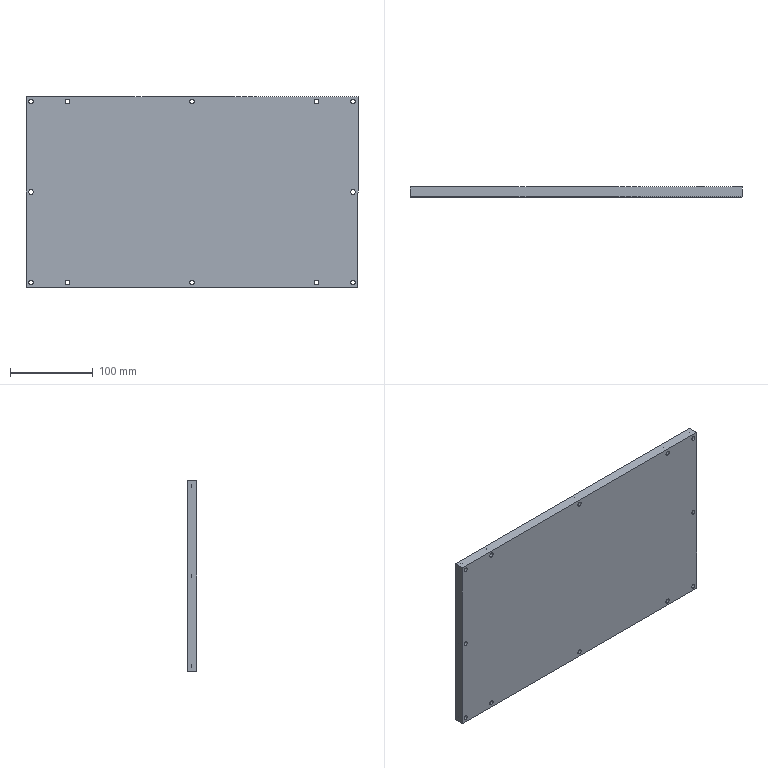Part | SolidWorks | features Extrusion 1, HoleWzd 1 | 1 solid | 66 faces | box 400 x 12 x 230 mm | volume 1097029 mm3 | cylinder 48 | plane 18 | commonest cylinder face diameters 5.5 x24 10 x24